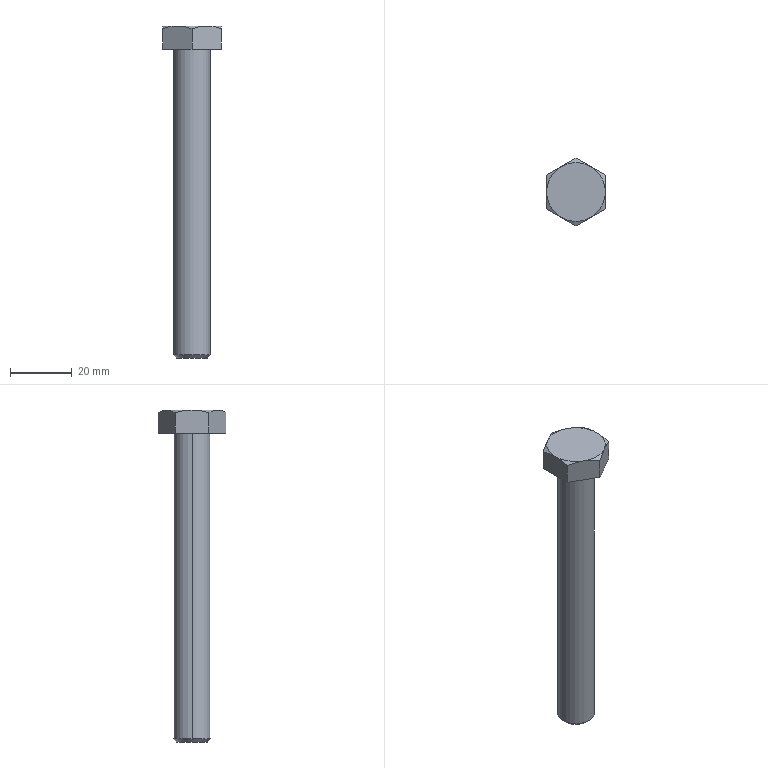Part | SolidWorks | features BaseBody 1 | 1 solid | 19 faces | box 19 x 21.939 x 107.5 mm | volume 13627 mm3 | plane 9 | cone 8 | cylinder 2 | commonest cylinder face diameters 12 x2
STEP:
#1=CARTESIAN_POINT('',(6.,0.,-98.927));
#2=VERTEX_POINT('',#1);
#3=CARTESIAN_POINT('',(-6.,0.,-98.927));
#4=VERTEX_POINT('',#3);
#5=CARTESIAN_POINT('',(0.,0.,-98.927));
#6=DIRECTION('',(0.,0.,1.));
#7=DIRECTION('',(1.,0.,0.));
#8=AXIS2_PLACEMENT_3D('',#5,#6,#7);
#9=CIRCLE('',#8,6.);
#10=EDGE_CURVE('',#2,#4,#9,.T.);
#11=ORIENTED_EDGE('',*,*,#10,.T.);
#12=CARTESIAN_POINT('',(-6.,0.,0.));
#13=VERTEX_POINT('',#12);
#14=CARTESIAN_POINT('',(-6.,0.,-100.));
#15=DIRECTION('',(0.,0.,1.));
#16=VECTOR('',#15,1000.);
#17=LINE('',#14,#16);
#18=EDGE_CURVE('',#4,#13,#17,.T.);
#19=ORIENTED_EDGE('',*,*,#18,.T.);
#20=CARTESIAN_POINT('',(6.,0.,0.));
#21=VERTEX_POINT('',#20);
#22=CARTESIAN_POINT('',(0.,0.,0.));
#23=DIRECTION('',(0.,0.,-1.));
#24=DIRECTION('',(1.,0.,0.));
#25=AXIS2_PLACEMENT_3D('',#22,#23,#24);
#26=CIRCLE('',#25,6.);
#27=EDGE_CURVE('',#13,#21,#26,.T.);
#28=ORIENTED_EDGE('',*,*,#27,.T.);
#29=CARTESIAN_POINT('',(6.,0.,-100.));
#30=DIRECTION('',(0.,0.,1.));
#31=VECTOR('',#30,1000.);
#32=LINE('',#29,#31);
#33=EDGE_CURVE('',#2,#21,#32,.T.);
#34=ORIENTED_EDGE('',*,*,#33,.F.);
#35=EDGE_LOOP('',(#11,#19,#28,#34));
#36=FACE_OUTER_BOUND('',#35,.T.);
#37=CARTESIAN_POINT('',(0.,0.,-100.));
#38=DIRECTION('',(0.,0.,1.));
#39=DIRECTION('',(1.,0.,0.));
#40=AXIS2_PLACEMENT_3D('',#37,#38,#39);
#41=CYLINDRICAL_SURFACE('',#40,6.);
#42=ADVANCED_FACE('',(#36),#41,.T.);
#43=CARTESIAN_POINT('',(4.927,0.,-100.));
#44=VERTEX_POINT('',#43);
#45=CARTESIAN_POINT('',(-4.927,0.,-100.));
#46=VERTEX_POINT('',#45);
#47=CARTESIAN_POINT('',(0.,0.,-100.));
#48=DIRECTION('',(0.,0.,1.));
#49=DIRECTION('',(1.,0.,0.));
#50=AXIS2_PLACEMENT_3D('',#47,#48,#49);
#51=CIRCLE('',#50,4.927);
#52=EDGE_CURVE('',#44,#46,#51,.T.);
#53=ORIENTED_EDGE('',*,*,#52,.T.);
#54=CARTESIAN_POINT('',(-6.,0.,-98.927));
#55=DIRECTION('',(-0.7071,0.,0.7071));
#56=VECTOR('',#55,1000.);
#57=LINE('',#54,#56);
#58=EDGE_CURVE('',#46,#4,#57,.T.);
#59=ORIENTED_EDGE('',*,*,#58,.T.);
#60=ORIENTED_EDGE('',*,*,#10,.F.);
#61=CARTESIAN_POINT('',(6.,0.,-98.927));
#62=DIRECTION('',(0.7071,0.,0.7071));
#63=VECTOR('',#62,1000.);
#64=LINE('',#61,#63);
#65=EDGE_CURVE('',#44,#2,#64,.T.);
#66=ORIENTED_EDGE('',*,*,#65,.F.);
#67=EDGE_LOOP('',(#53,#59,#60,#66));
#68=FACE_OUTER_BOUND('',#67,.T.);
#69=CARTESIAN_POINT('',(0.,0.,-98.927));
#70=DIRECTION('',(0.,0.,1.));
#71=DIRECTION('',(1.,0.,0.));
#72=AXIS2_PLACEMENT_3D('',#69,#70,#71);
#73=CONICAL_SURFACE('',#72,6.,0.7854);
#74=ADVANCED_FACE('',(#68),#73,.T.);
#75=ORIENTED_EDGE('',*,*,#18,.F.);
#76=CARTESIAN_POINT('',(0.,0.,-98.927));
#77=DIRECTION('',(0.,0.,1.));
#78=DIRECTION('',(1.,0.,0.));
#79=AXIS2_PLACEMENT_3D('',#76,#77,#78);
#80=CIRCLE('',#79,6.);
#81=EDGE_CURVE('',#4,#2,#80,.T.);
#82=ORIENTED_EDGE('',*,*,#81,.T.);
#83=ORIENTED_EDGE('',*,*,#33,.T.);
#84=CARTESIAN_POINT('',(0.,0.,0.));
#85=DIRECTION('',(0.,0.,-1.));
#86=DIRECTION('',(1.,0.,0.));
#87=AXIS2_PLACEMENT_3D('',#84,#85,#86);
#88=CIRCLE('',#87,6.);
#89=EDGE_CURVE('',#21,#13,#88,.T.);
#90=ORIENTED_EDGE('',*,*,#89,.T.);
#91=EDGE_LOOP('',(#75,#82,#83,#90));
#92=FACE_OUTER_BOUND('',#91,.T.);
#93=CARTESIAN_POINT('',(0.,0.,-100.));
#94=DIRECTION('',(0.,0.,1.));
#95=DIRECTION('',(1.,0.,0.));
#96=AXIS2_PLACEMENT_3D('',#93,#94,#95);
#97=CYLINDRICAL_SURFACE('',#96,6.);
#98=ADVANCED_FACE('',(#92),#97,.T.);
#99=ORIENTED_EDGE('',*,*,#89,.F.);
#100=ORIENTED_EDGE('',*,*,#27,.F.);
#101=EDGE_LOOP('',(#99,#100));
#102=FACE_BOUND('',#101,.T.);
#103=CARTESIAN_POINT('',(-9.5,5.485,0.));
#104=VERTEX_POINT('',#103);
#105=CARTESIAN_POINT('',(-9.5,-5.485,0.));
#106=VERTEX_POINT('',#105);
#107=CARTESIAN_POINT('',(-9.5,0.,0.));
#108=DIRECTION('',(0.,-1.,0.));
#109=VECTOR('',#108,1000.);
#110=LINE('',#107,#109);
#111=EDGE_CURVE('',#104,#106,#110,.T.);
#112=ORIENTED_EDGE('',*,*,#111,.F.);
#113=CARTESIAN_POINT('',(0.,10.97,0.));
#114=VERTEX_POINT('',#113);
#115=CARTESIAN_POINT('',(0.,10.97,0.));
#116=DIRECTION('',(-0.866,-0.5,0.));
#117=VECTOR('',#116,1000.);
#118=LINE('',#115,#117);
#119=EDGE_CURVE('',#114,#104,#118,.T.);
#120=ORIENTED_EDGE('',*,*,#119,.F.);
#121=CARTESIAN_POINT('',(9.5,5.485,0.));
#122=VERTEX_POINT('',#121);
#123=CARTESIAN_POINT('',(9.5,5.485,0.));
#124=DIRECTION('',(-0.866,0.5,0.));
#125=VECTOR('',#124,1000.);
#126=LINE('',#123,#125);
#127=EDGE_CURVE('',#122,#114,#126,.T.);
#128=ORIENTED_EDGE('',*,*,#127,.F.);
#129=CARTESIAN_POINT('',(9.5,-5.485,0.));
#130=VERTEX_POINT('',#129);
#131=CARTESIAN_POINT('',(9.5,0.,0.));
#132=DIRECTION('',(0.,1.,0.));
#133=VECTOR('',#132,1000.);
#134=LINE('',#131,#133);
#135=EDGE_CURVE('',#130,#122,#134,.T.);
#136=ORIENTED_EDGE('',*,*,#135,.F.);
#137=CARTESIAN_POINT('',(0.,-10.97,0.));
#138=VERTEX_POINT('',#137);
#139=CARTESIAN_POINT('',(0.,-10.97,0.));
#140=DIRECTION('',(0.866,0.5,0.));
#141=VECTOR('',#140,1000.);
#142=LINE('',#139,#141);
#143=EDGE_CURVE('',#138,#130,#142,.T.);
#144=ORIENTED_EDGE('',*,*,#143,.F.);
#145=CARTESIAN_POINT('',(-9.5,-5.485,0.));
#146=DIRECTION('',(0.866,-0.5,0.));
#147=VECTOR('',#146,1000.);
#148=LINE('',#145,#147);
#149=EDGE_CURVE('',#106,#138,#148,.T.);
#150=ORIENTED_EDGE('',*,*,#149,.F.);
#151=EDGE_LOOP('',(#112,#120,#128,#136,#144,#150));
#152=FACE_OUTER_BOUND('',#151,.T.);
#153=CARTESIAN_POINT('',(0.,0.,0.));
#154=DIRECTION('',(0.,0.,1.));
#155=DIRECTION('',(1.,0.,0.));
#156=AXIS2_PLACEMENT_3D('',#153,#154,#155);
#157=PLANE('',#156);
#158=ADVANCED_FACE('',(#102,#152),#157,.F.);
#159=ORIENTED_EDGE('',*,*,#58,.F.);
#160=CARTESIAN_POINT('',(0.,0.,-100.));
#161=DIRECTION('',(0.,0.,1.));
#162=DIRECTION('',(1.,0.,0.));
#163=AXIS2_PLACEMENT_3D('',#160,#161,#162);
#164=CIRCLE('',#163,4.927);
#165=EDGE_CURVE('',#46,#44,#164,.T.);
#166=ORIENTED_EDGE('',*,*,#165,.T.);
#167=ORIENTED_EDGE('',*,*,#65,.T.);
#168=ORIENTED_EDGE('',*,*,#81,.F.);
#169=EDGE_LOOP('',(#159,#166,#167,#168));
#170=FACE_OUTER_BOUND('',#169,.T.);
#171=CARTESIAN_POINT('',(0.,0.,-98.927));
#172=DIRECTION('',(0.,0.,1.));
#173=DIRECTION('',(1.,0.,0.));
#174=AXIS2_PLACEMENT_3D('',#171,#172,#173);
#175=CONICAL_SURFACE('',#174,6.,0.7854);
#176=ADVANCED_FACE('',(#170),#175,.T.);
#177=CARTESIAN_POINT('',(-4.75,-8.227,7.5));
#178=VERTEX_POINT('',#177);
#179=CARTESIAN_POINT('',(0.,-10.97,6.651));
#180=VERTEX_POINT('',#179);
#181=CARTESIAN_POINT('',(-4.75,-8.227,7.5));
#182=CARTESIAN_POINT('',(-3.939,-8.695,7.5));
#183=CARTESIAN_POINT('',(-3.14,-9.157,7.419));
#184=CARTESIAN_POINT('',(-1.558,-10.07,7.123));
#185=CARTESIAN_POINT('',(-0.776,-10.522,6.91));
#186=CARTESIAN_POINT('',(0.,-10.97,6.651));
#187=B_SPLINE_CURVE_WITH_KNOTS('',3,(#181,#182,#183,#184,#185,#186),.UNSPECIFIED.,.F.,.F.,(4,2,4),(0.,0.002775,0.00555),.UNSPECIFIED.);
#188=EDGE_CURVE('',#178,#180,#187,.T.);
#189=ORIENTED_EDGE('',*,*,#188,.F.);
#190=CARTESIAN_POINT('',(-9.5,-5.485,6.651));
#191=VERTEX_POINT('',#190);
#192=CARTESIAN_POINT('',(-9.5,-5.485,6.651));
#193=CARTESIAN_POINT('',(-8.724,-5.933,6.91));
#194=CARTESIAN_POINT('',(-7.942,-6.384,7.123));
#195=CARTESIAN_POINT('',(-6.36,-7.298,7.419));
#196=CARTESIAN_POINT('',(-5.561,-7.759,7.5));
#197=CARTESIAN_POINT('',(-4.75,-8.227,7.5));
#198=B_SPLINE_CURVE_WITH_KNOTS('',3,(#192,#193,#194,#195,#196,#197),.UNSPECIFIED.,.F.,.F.,(4,2,4),(0.,0.002775,0.00555),.UNSPECIFIED.);
#199=EDGE_CURVE('',#191,#178,#198,.T.);
#200=ORIENTED_EDGE('',*,*,#199,.F.);
#201=CARTESIAN_POINT('',(-9.5,-5.485,7.5));
#202=DIRECTION('',(0.,0.,1.));
#203=VECTOR('',#202,1000.);
#204=LINE('',#201,#203);
#205=EDGE_CURVE('',#106,#191,#204,.T.);
#206=ORIENTED_EDGE('',*,*,#205,.F.);
#207=ORIENTED_EDGE('',*,*,#149,.T.);
#208=CARTESIAN_POINT('',(0.,-10.97,7.5));
#209=DIRECTION('',(0.,0.,-1.));
#210=VECTOR('',#209,1000.);
#211=LINE('',#208,#210);
#212=EDGE_CURVE('',#180,#138,#211,.T.);
#213=ORIENTED_EDGE('',*,*,#212,.F.);
#214=EDGE_LOOP('',(#189,#200,#206,#207,#213));
#215=FACE_OUTER_BOUND('',#214,.T.);
#216=CARTESIAN_POINT('',(-9.5,-5.485,7.5));
#217=DIRECTION('',(0.5,0.866,0.));
#218=DIRECTION('',(-0.866,0.5,0.));
#219=AXIS2_PLACEMENT_3D('',#216,#217,#218);
#220=PLANE('',#219);
#221=ADVANCED_FACE('',(#215),#220,.F.);
#222=CARTESIAN_POINT('',(-9.5,0.,7.5));
#223=VERTEX_POINT('',#222);
#224=CARTESIAN_POINT('',(-9.5,0.,7.5));
#225=CARTESIAN_POINT('',(-9.5,-0.936,7.5));
#226=CARTESIAN_POINT('',(-9.5,-1.859,7.419));
#227=CARTESIAN_POINT('',(-9.5,-3.686,7.123));
#228=CARTESIAN_POINT('',(-9.5,-4.589,6.91));
#229=CARTESIAN_POINT('',(-9.5,-5.485,6.651));
#230=B_SPLINE_CURVE_WITH_KNOTS('',3,(#224,#225,#226,#227,#228,#229),.UNSPECIFIED.,.F.,.F.,(4,2,4),(0.,0.002775,0.00555),.UNSPECIFIED.);
#231=EDGE_CURVE('',#223,#191,#230,.T.);
#232=ORIENTED_EDGE('',*,*,#231,.F.);
#233=CARTESIAN_POINT('',(-9.5,5.485,6.651));
#234=VERTEX_POINT('',#233);
#235=CARTESIAN_POINT('',(-9.5,5.485,6.651));
#236=CARTESIAN_POINT('',(-9.5,4.589,6.91));
#237=CARTESIAN_POINT('',(-9.5,3.686,7.123));
#238=CARTESIAN_POINT('',(-9.5,1.859,7.419));
#239=CARTESIAN_POINT('',(-9.5,0.936,7.5));
#240=CARTESIAN_POINT('',(-9.5,0.,7.5));
#241=B_SPLINE_CURVE_WITH_KNOTS('',3,(#235,#236,#237,#238,#239,#240),.UNSPECIFIED.,.F.,.F.,(4,2,4),(0.,0.002775,0.00555),.UNSPECIFIED.);
#242=EDGE_CURVE('',#234,#223,#241,.T.);
#243=ORIENTED_EDGE('',*,*,#242,.F.);
#244=CARTESIAN_POINT('',(-9.5,5.485,7.5));
#245=DIRECTION('',(0.,0.,1.));
#246=VECTOR('',#245,1000.);
#247=LINE('',#244,#246);
#248=EDGE_CURVE('',#104,#234,#247,.T.);
#249=ORIENTED_EDGE('',*,*,#248,.F.);
#250=ORIENTED_EDGE('',*,*,#111,.T.);
#251=ORIENTED_EDGE('',*,*,#205,.T.);
#252=EDGE_LOOP('',(#232,#243,#249,#250,#251));
#253=FACE_OUTER_BOUND('',#252,.T.);
#254=CARTESIAN_POINT('',(-9.5,5.485,7.5));
#255=DIRECTION('',(1.,0.,0.));
#256=DIRECTION('',(0.,0.,-1.));
#257=AXIS2_PLACEMENT_3D('',#254,#255,#256);
#258=PLANE('',#257);
#259=ADVANCED_FACE('',(#253),#258,.F.);
#260=CARTESIAN_POINT('',(-4.75,8.227,7.5));
#261=VERTEX_POINT('',#260);
#262=CARTESIAN_POINT('',(-4.75,8.227,7.5));
#263=CARTESIAN_POINT('',(-5.561,7.759,7.5));
#264=CARTESIAN_POINT('',(-6.36,7.298,7.419));
#265=CARTESIAN_POINT('',(-7.942,6.384,7.123));
#266=CARTESIAN_POINT('',(-8.724,5.933,6.91));
#267=CARTESIAN_POINT('',(-9.5,5.485,6.651));
#268=B_SPLINE_CURVE_WITH_KNOTS('',3,(#262,#263,#264,#265,#266,#267),.UNSPECIFIED.,.F.,.F.,(4,2,4),(0.,0.002775,0.00555),.UNSPECIFIED.);
#269=EDGE_CURVE('',#261,#234,#268,.T.);
#270=ORIENTED_EDGE('',*,*,#269,.F.);
#271=CARTESIAN_POINT('',(0.,10.97,6.651));
#272=VERTEX_POINT('',#271);
#273=CARTESIAN_POINT('',(0.,10.97,6.651));
#274=CARTESIAN_POINT('',(-0.776,10.522,6.91));
#275=CARTESIAN_POINT('',(-1.558,10.07,7.123));
#276=CARTESIAN_POINT('',(-3.14,9.157,7.419));
#277=CARTESIAN_POINT('',(-3.939,8.695,7.5));
#278=CARTESIAN_POINT('',(-4.75,8.227,7.5));
#279=B_SPLINE_CURVE_WITH_KNOTS('',3,(#273,#274,#275,#276,#277,#278),.UNSPECIFIED.,.F.,.F.,(4,2,4),(0.,0.002775,0.00555),.UNSPECIFIED.);
#280=EDGE_CURVE('',#272,#261,#279,.T.);
#281=ORIENTED_EDGE('',*,*,#280,.F.);
#282=CARTESIAN_POINT('',(0.,10.97,7.5));
#283=DIRECTION('',(0.,0.,1.));
#284=VECTOR('',#283,1000.);
#285=LINE('',#282,#284);
#286=EDGE_CURVE('',#114,#272,#285,.T.);
#287=ORIENTED_EDGE('',*,*,#286,.F.);
#288=ORIENTED_EDGE('',*,*,#119,.T.);
#289=ORIENTED_EDGE('',*,*,#248,.T.);
#290=EDGE_LOOP('',(#270,#281,#287,#288,#289));
#291=FACE_OUTER_BOUND('',#290,.T.);
#292=CARTESIAN_POINT('',(0.,10.97,7.5));
#293=DIRECTION('',(0.5,-0.866,0.));
#294=DIRECTION('',(0.866,0.5,0.));
#295=AXIS2_PLACEMENT_3D('',#292,#293,#294);
#296=PLANE('',#295);
#297=ADVANCED_FACE('',(#291),#296,.F.);
#298=CARTESIAN_POINT('',(4.75,8.227,7.5));
#299=VERTEX_POINT('',#298);
#300=CARTESIAN_POINT('',(4.75,8.227,7.5));
#301=CARTESIAN_POINT('',(3.939,8.695,7.5));
#302=CARTESIAN_POINT('',(3.14,9.157,7.419));
#303=CARTESIAN_POINT('',(1.558,10.07,7.123));
#304=CARTESIAN_POINT('',(0.776,10.522,6.91));
#305=CARTESIAN_POINT('',(0.,10.97,6.651));
#306=B_SPLINE_CURVE_WITH_KNOTS('',3,(#300,#301,#302,#303,#304,#305),.UNSPECIFIED.,.F.,.F.,(4,2,4),(0.,0.002775,0.00555),.UNSPECIFIED.);
#307=EDGE_CURVE('',#299,#272,#306,.T.);
#308=ORIENTED_EDGE('',*,*,#307,.F.);
#309=CARTESIAN_POINT('',(9.5,5.485,6.651));
#310=VERTEX_POINT('',#309);
#311=CARTESIAN_POINT('',(9.5,5.485,6.651));
#312=CARTESIAN_POINT('',(8.724,5.933,6.91));
#313=CARTESIAN_POINT('',(7.942,6.384,7.123));
#314=CARTESIAN_POINT('',(6.36,7.298,7.419));
#315=CARTESIAN_POINT('',(5.561,7.759,7.5));
#316=CARTESIAN_POINT('',(4.75,8.227,7.5));
#317=B_SPLINE_CURVE_WITH_KNOTS('',3,(#311,#312,#313,#314,#315,#316),.UNSPECIFIED.,.F.,.F.,(4,2,4),(0.,0.002775,0.00555),.UNSPECIFIED.);
#318=EDGE_CURVE('',#310,#299,#317,.T.);
#319=ORIENTED_EDGE('',*,*,#318,.F.);
#320=CARTESIAN_POINT('',(9.5,5.485,7.5));
#321=DIRECTION('',(0.,0.,1.));
#322=VECTOR('',#321,1000.);
#323=LINE('',#320,#322);
#324=EDGE_CURVE('',#122,#310,#323,.T.);
#325=ORIENTED_EDGE('',*,*,#324,.F.);
#326=ORIENTED_EDGE('',*,*,#127,.T.);
#327=ORIENTED_EDGE('',*,*,#286,.T.);
#328=EDGE_LOOP('',(#308,#319,#325,#326,#327));
#329=FACE_OUTER_BOUND('',#328,.T.);
#330=CARTESIAN_POINT('',(9.5,5.485,7.5));
#331=DIRECTION('',(-0.5,-0.866,0.));
#332=DIRECTION('',(0.866,-0.5,0.));
#333=AXIS2_PLACEMENT_3D('',#330,#331,#332);
#334=PLANE('',#333);
#335=ADVANCED_FACE('',(#329),#334,.F.);
#336=CARTESIAN_POINT('',(9.5,0.,7.5));
#337=VERTEX_POINT('',#336);
#338=CARTESIAN_POINT('',(9.5,0.,7.5));
#339=CARTESIAN_POINT('',(9.5,0.936,7.5));
#340=CARTESIAN_POINT('',(9.5,1.859,7.419));
#341=CARTESIAN_POINT('',(9.5,3.686,7.123));
#342=CARTESIAN_POINT('',(9.5,4.589,6.91));
#343=CARTESIAN_POINT('',(9.5,5.485,6.651));
#344=B_SPLINE_CURVE_WITH_KNOTS('',3,(#338,#339,#340,#341,#342,#343),.UNSPECIFIED.,.F.,.F.,(4,2,4),(0.,0.002775,0.00555),.UNSPECIFIED.);
#345=EDGE_CURVE('',#337,#310,#344,.T.);
#346=ORIENTED_EDGE('',*,*,#345,.F.);
#347=CARTESIAN_POINT('',(9.5,-5.485,6.651));
#348=VERTEX_POINT('',#347);
#349=CARTESIAN_POINT('',(9.5,-5.485,6.651));
#350=CARTESIAN_POINT('',(9.5,-4.589,6.91));
#351=CARTESIAN_POINT('',(9.5,-3.686,7.123));
#352=CARTESIAN_POINT('',(9.5,-1.859,7.419));
#353=CARTESIAN_POINT('',(9.5,-0.936,7.5));
#354=CARTESIAN_POINT('',(9.5,0.,7.5));
#355=B_SPLINE_CURVE_WITH_KNOTS('',3,(#349,#350,#351,#352,#353,#354),.UNSPECIFIED.,.F.,.F.,(4,2,4),(0.,0.002775,0.00555),.UNSPECIFIED.);
#356=EDGE_CURVE('',#348,#337,#355,.T.);
#357=ORIENTED_EDGE('',*,*,#356,.F.);
#358=CARTESIAN_POINT('',(9.5,-5.485,7.5));
#359=DIRECTION('',(0.,0.,1.));
#360=VECTOR('',#359,1000.);
#361=LINE('',#358,#360);
#362=EDGE_CURVE('',#130,#348,#361,.T.);
#363=ORIENTED_EDGE('',*,*,#362,.F.);
#364=ORIENTED_EDGE('',*,*,#135,.T.);
#365=ORIENTED_EDGE('',*,*,#324,.T.);
#366=EDGE_LOOP('',(#346,#357,#363,#364,#365));
#367=FACE_OUTER_BOUND('',#366,.T.);
#368=CARTESIAN_POINT('',(9.5,-5.485,7.5));
#369=DIRECTION('',(-1.,0.,0.));
#370=DIRECTION('',(0.,0.,1.));
#371=AXIS2_PLACEMENT_3D('',#368,#369,#370);
#372=PLANE('',#371);
#373=ADVANCED_FACE('',(#367),#372,.F.);
#374=CARTESIAN_POINT('',(4.75,-8.227,7.5));
#375=VERTEX_POINT('',#374);
#376=CARTESIAN_POINT('',(4.75,-8.227,7.5));
#377=CARTESIAN_POINT('',(5.561,-7.759,7.5));
#378=CARTESIAN_POINT('',(6.36,-7.298,7.419));
#379=CARTESIAN_POINT('',(7.942,-6.384,7.123));
#380=CARTESIAN_POINT('',(8.724,-5.933,6.91));
#381=CARTESIAN_POINT('',(9.5,-5.485,6.651));
#382=B_SPLINE_CURVE_WITH_KNOTS('',3,(#376,#377,#378,#379,#380,#381),.UNSPECIFIED.,.F.,.F.,(4,2,4),(0.,0.002775,0.00555),.UNSPECIFIED.);
#383=EDGE_CURVE('',#375,#348,#382,.T.);
#384=ORIENTED_EDGE('',*,*,#383,.F.);
#385=CARTESIAN_POINT('',(0.,-10.97,6.651));
#386=CARTESIAN_POINT('',(0.776,-10.522,6.91));
#387=CARTESIAN_POINT('',(1.558,-10.07,7.123));
#388=CARTESIAN_POINT('',(3.14,-9.157,7.419));
#389=CARTESIAN_POINT('',(3.939,-8.695,7.5));
#390=CARTESIAN_POINT('',(4.75,-8.227,7.5));
#391=B_SPLINE_CURVE_WITH_KNOTS('',3,(#385,#386,#387,#388,#389,#390),.UNSPECIFIED.,.F.,.F.,(4,2,4),(0.,0.002775,0.00555),.UNSPECIFIED.);
#392=EDGE_CURVE('',#180,#375,#391,.T.);
#393=ORIENTED_EDGE('',*,*,#392,.F.);
#394=ORIENTED_EDGE('',*,*,#212,.T.);
#395=ORIENTED_EDGE('',*,*,#143,.T.);
#396=ORIENTED_EDGE('',*,*,#362,.T.);
#397=EDGE_LOOP('',(#384,#393,#394,#395,#396));
#398=FACE_OUTER_BOUND('',#397,.T.);
#399=CARTESIAN_POINT('',(0.,-10.97,7.5));
#400=DIRECTION('',(-0.5,0.866,0.));
#401=DIRECTION('',(-0.866,-0.5,0.));
#402=AXIS2_PLACEMENT_3D('',#399,#400,#401);
#403=PLANE('',#402);
#404=ADVANCED_FACE('',(#398),#403,.F.);
#405=ORIENTED_EDGE('',*,*,#52,.F.);
#406=ORIENTED_EDGE('',*,*,#165,.F.);
#407=EDGE_LOOP('',(#405,#406));
#408=FACE_OUTER_BOUND('',#407,.T.);
#409=CARTESIAN_POINT('',(0.,4.927,-100.));
#410=DIRECTION('',(0.,0.,1.));
#411=DIRECTION('',(1.,0.,0.));
#412=AXIS2_PLACEMENT_3D('',#409,#410,#411);
#413=PLANE('',#412);
#414=ADVANCED_FACE('',(#408),#413,.F.);
#415=ORIENTED_EDGE('',*,*,#188,.T.);
#416=ORIENTED_EDGE('',*,*,#392,.T.);
#417=CARTESIAN_POINT('',(0.,0.,7.5));
#418=DIRECTION('',(0.,0.,-1.));
#419=DIRECTION('',(-1.,0.,0.));
#420=AXIS2_PLACEMENT_3D('',#417,#418,#419);
#421=CIRCLE('',#420,9.5);
#422=EDGE_CURVE('',#375,#178,#421,.T.);
#423=ORIENTED_EDGE('',*,*,#422,.T.);
#424=EDGE_LOOP('',(#415,#416,#423));
#425=FACE_OUTER_BOUND('',#424,.T.);
#426=CARTESIAN_POINT('',(0.,0.,6.646));
#427=DIRECTION('',(0.,0.,-1.));
#428=DIRECTION('',(-1.,0.,0.));
#429=AXIS2_PLACEMENT_3D('',#426,#427,#428);
#430=CONICAL_SURFACE('',#429,10.978,1.047);
#431=ADVANCED_FACE('',(#425),#430,.T.);
#432=ORIENTED_EDGE('',*,*,#231,.T.);
#433=ORIENTED_EDGE('',*,*,#199,.T.);
#434=CARTESIAN_POINT('',(0.,0.,7.5));
#435=DIRECTION('',(0.,0.,-1.));
#436=DIRECTION('',(0.,1.,0.));
#437=AXIS2_PLACEMENT_3D('',#434,#435,#436);
#438=CIRCLE('',#437,9.5);
#439=EDGE_CURVE('',#178,#223,#438,.T.);
#440=ORIENTED_EDGE('',*,*,#439,.T.);
#441=EDGE_LOOP('',(#432,#433,#440));
#442=FACE_OUTER_BOUND('',#441,.T.);
#443=CARTESIAN_POINT('',(0.,0.,6.646));
#444=DIRECTION('',(0.,0.,-1.));
#445=DIRECTION('',(0.,1.,0.));
#446=AXIS2_PLACEMENT_3D('',#443,#444,#445);
#447=CONICAL_SURFACE('',#446,10.978,1.047);
#448=ADVANCED_FACE('',(#442),#447,.T.);
#449=CARTESIAN_POINT('',(0.,0.,7.5));
#450=DIRECTION('',(0.,0.,-1.));
#451=DIRECTION('',(0.,1.,0.));
#452=AXIS2_PLACEMENT_3D('',#449,#450,#451);
#453=CIRCLE('',#452,9.5);
#454=EDGE_CURVE('',#223,#261,#453,.T.);
#455=ORIENTED_EDGE('',*,*,#454,.T.);
#456=ORIENTED_EDGE('',*,*,#269,.T.);
#457=ORIENTED_EDGE('',*,*,#242,.T.);
#458=EDGE_LOOP('',(#455,#456,#457));
#459=FACE_OUTER_BOUND('',#458,.T.);
#460=CARTESIAN_POINT('',(0.,0.,6.646));
#461=DIRECTION('',(0.,0.,-1.));
#462=DIRECTION('',(0.,1.,0.));
#463=AXIS2_PLACEMENT_3D('',#460,#461,#462);
#464=CONICAL_SURFACE('',#463,10.978,1.047);
#465=ADVANCED_FACE('',(#459),#464,.T.);
#466=ORIENTED_EDGE('',*,*,#280,.T.);
#467=CARTESIAN_POINT('',(0.,0.,7.5));
#468=DIRECTION('',(0.,0.,-1.));
#469=DIRECTION('',(-1.,0.,0.));
#470=AXIS2_PLACEMENT_3D('',#467,#468,#469);
#471=CIRCLE('',#470,9.5);
#472=EDGE_CURVE('',#261,#299,#471,.T.);
#473=ORIENTED_EDGE('',*,*,#472,.T.);
#474=ORIENTED_EDGE('',*,*,#307,.T.);
#475=EDGE_LOOP('',(#466,#473,#474));
#476=FACE_OUTER_BOUND('',#475,.T.);
#477=CARTESIAN_POINT('',(0.,0.,6.646));
#478=DIRECTION('',(0.,0.,-1.));
#479=DIRECTION('',(-1.,0.,0.));
#480=AXIS2_PLACEMENT_3D('',#477,#478,#479);
#481=CONICAL_SURFACE('',#480,10.978,1.047);
#482=ADVANCED_FACE('',(#476),#481,.T.);
#483=CARTESIAN_POINT('',(0.,0.,7.5));
#484=DIRECTION('',(0.,0.,-1.));
#485=DIRECTION('',(0.,1.,0.));
#486=AXIS2_PLACEMENT_3D('',#483,#484,#485);
#487=CIRCLE('',#486,9.5);
#488=EDGE_CURVE('',#299,#337,#487,.T.);
#489=ORIENTED_EDGE('',*,*,#488,.T.);
#490=ORIENTED_EDGE('',*,*,#345,.T.);
#491=ORIENTED_EDGE('',*,*,#318,.T.);
#492=EDGE_LOOP('',(#489,#490,#491));
#493=FACE_OUTER_BOUND('',#492,.T.);
#494=CARTESIAN_POINT('',(0.,0.,6.646));
#495=DIRECTION('',(0.,0.,-1.));
#496=DIRECTION('',(0.,1.,0.));
#497=AXIS2_PLACEMENT_3D('',#494,#495,#496);
#498=CONICAL_SURFACE('',#497,10.978,1.047);
#499=ADVANCED_FACE('',(#493),#498,.T.);
#500=ORIENTED_EDGE('',*,*,#383,.T.);
#501=ORIENTED_EDGE('',*,*,#356,.T.);
#502=CARTESIAN_POINT('',(0.,0.,7.5));
#503=DIRECTION('',(0.,0.,-1.));
#504=DIRECTION('',(0.,1.,0.));
#505=AXIS2_PLACEMENT_3D('',#502,#503,#504);
#506=CIRCLE('',#505,9.5);
#507=EDGE_CURVE('',#337,#375,#506,.T.);
#508=ORIENTED_EDGE('',*,*,#507,.T.);
#509=EDGE_LOOP('',(#500,#501,#508));
#510=FACE_OUTER_BOUND('',#509,.T.);
#511=CARTESIAN_POINT('',(0.,0.,6.646));
#512=DIRECTION('',(0.,0.,-1.));
#513=DIRECTION('',(0.,1.,0.));
#514=AXIS2_PLACEMENT_3D('',#511,#512,#513);
#515=CONICAL_SURFACE('',#514,10.978,1.047);
#516=ADVANCED_FACE('',(#510),#515,.T.);
#517=ORIENTED_EDGE('',*,*,#454,.F.);
#518=ORIENTED_EDGE('',*,*,#439,.F.);
#519=ORIENTED_EDGE('',*,*,#422,.F.);
#520=ORIENTED_EDGE('',*,*,#507,.F.);
#521=ORIENTED_EDGE('',*,*,#488,.F.);
#522=ORIENTED_EDGE('',*,*,#472,.F.);
#523=EDGE_LOOP('',(#517,#518,#519,#520,#521,#522));
#524=FACE_OUTER_BOUND('',#523,.T.);
#525=CARTESIAN_POINT('',(0.,0.,7.5));
#526=DIRECTION('',(0.,0.,1.));
#527=DIRECTION('',(1.,0.,0.));
#528=AXIS2_PLACEMENT_3D('',#525,#526,#527);
#529=PLANE('',#528);
#530=ADVANCED_FACE('',(#524),#529,.T.);
#531=CLOSED_SHELL('',(#42,#74,#98,#158,#176,#221,#259,#297,#335,#373,#404,#414,#431,#448,#465,#482,#499,#516,#530));
#532=MANIFOLD_SOLID_BREP('',#531);
#533=CARTESIAN_POINT('',(0.,0.,0.));
#534=DIRECTION('',(0.,0.,1.));
#535=DIRECTION('',(1.,0.,0.));
#536=AXIS2_PLACEMENT_3D('',#533,#534,#535);
#537=(LENGTH_UNIT()NAMED_UNIT(*)SI_UNIT(.MILLI.,.METRE.));
#538=UNCERTAINTY_MEASURE_WITH_UNIT(LENGTH_MEASURE(0.00001),#537,'','');
#539=(NAMED_UNIT(*)PLANE_ANGLE_UNIT()SI_UNIT($,.RADIAN.));
#540=(NAMED_UNIT(*)SI_UNIT($,.STERADIAN.)SOLID_ANGLE_UNIT());
#541=(GEOMETRIC_REPRESENTATION_CONTEXT(3)GLOBAL_UNCERTAINTY_ASSIGNED_CONTEXT((#538))GLOBAL_UNIT_ASSIGNED_CONTEXT((#537,#539,#540))REPRESENTATION_CONTEXT('',''));
#542=ADVANCED_BREP_SHAPE_REPRESENTATION('',(#532,#536),#541);